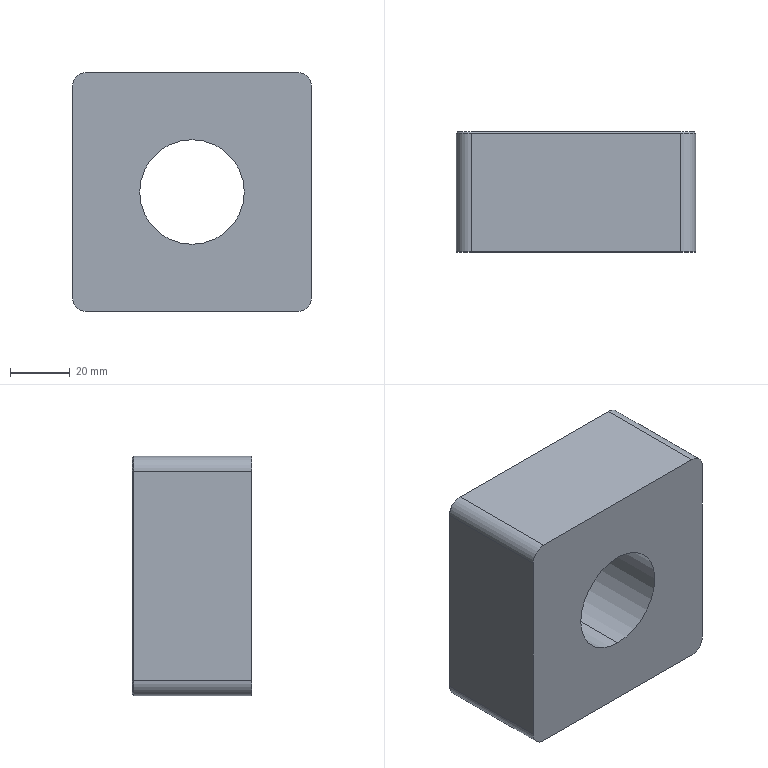Part | SolidWorks | features Chamfer 1, Extrusion 1, Fillet 1, HoleWzd 1 | 1 solid | 20 faces | box 80 x 40 x 80 mm | volume 216618 mm3 | plane 10 | cylinder 6 | cone 4 | commonest cylinder face diameters 10 x4 35 x2
STEP:
#1=CARTESIAN_POINT('',(0.,-25.,-17.5));
#2=VERTEX_POINT('',#1);
#3=CARTESIAN_POINT('',(0.,-25.,17.5));
#4=VERTEX_POINT('',#3);
#5=CARTESIAN_POINT('',(0.,-25.,0.));
#6=DIRECTION('',(0.,1.,0.));
#7=DIRECTION('',(0.,0.,1.));
#8=AXIS2_PLACEMENT_3D('',#5,#6,#7);
#9=CIRCLE('',#8,17.5);
#10=EDGE_CURVE('',#2,#4,#9,.T.);
#11=ORIENTED_EDGE('',*,*,#10,.F.);
#12=CARTESIAN_POINT('',(0.,15.,-17.5));
#13=VERTEX_POINT('',#12);
#14=CARTESIAN_POINT('',(0.,15.,-17.5));
#15=DIRECTION('',(0.,1.,0.));
#16=VECTOR('',#15,1000.);
#17=LINE('',#14,#16);
#18=EDGE_CURVE('',#2,#13,#17,.T.);
#19=ORIENTED_EDGE('',*,*,#18,.T.);
#20=CARTESIAN_POINT('',(0.,15.,17.5));
#21=VERTEX_POINT('',#20);
#22=CARTESIAN_POINT('',(0.,15.,0.));
#23=DIRECTION('',(0.,1.,0.));
#24=DIRECTION('',(0.,0.,1.));
#25=AXIS2_PLACEMENT_3D('',#22,#23,#24);
#26=CIRCLE('',#25,17.5);
#27=EDGE_CURVE('',#13,#21,#26,.T.);
#28=ORIENTED_EDGE('',*,*,#27,.T.);
#29=CARTESIAN_POINT('',(0.,15.,17.5));
#30=DIRECTION('',(0.,1.,0.));
#31=VECTOR('',#30,1000.);
#32=LINE('',#29,#31);
#33=EDGE_CURVE('',#4,#21,#32,.T.);
#34=ORIENTED_EDGE('',*,*,#33,.F.);
#35=EDGE_LOOP('',(#11,#19,#28,#34));
#36=FACE_OUTER_BOUND('',#35,.T.);
#37=CARTESIAN_POINT('',(0.,15.,0.));
#38=DIRECTION('',(0.,1.,0.));
#39=DIRECTION('',(0.,0.,1.));
#40=AXIS2_PLACEMENT_3D('',#37,#38,#39);
#41=CYLINDRICAL_SURFACE('',#40,17.5);
#42=ADVANCED_FACE('',(#36),#41,.F.);
#43=CARTESIAN_POINT('',(-40.,-25.,35.));
#44=VERTEX_POINT('',#43);
#45=CARTESIAN_POINT('',(-40.,14.5,35.));
#46=VERTEX_POINT('',#45);
#47=CARTESIAN_POINT('',(-40.,-25.,35.));
#48=DIRECTION('',(0.,1.,0.));
#49=VECTOR('',#48,1000.);
#50=LINE('',#47,#49);
#51=EDGE_CURVE('',#44,#46,#50,.T.);
#52=ORIENTED_EDGE('',*,*,#51,.T.);
#53=CARTESIAN_POINT('',(-40.,14.5,-35.));
#54=VERTEX_POINT('',#53);
#55=CARTESIAN_POINT('',(-40.,14.5,-40.));
#56=DIRECTION('',(0.,0.,-1.));
#57=VECTOR('',#56,1000.);
#58=LINE('',#55,#57);
#59=EDGE_CURVE('',#46,#54,#58,.T.);
#60=ORIENTED_EDGE('',*,*,#59,.T.);
#61=CARTESIAN_POINT('',(-40.,-25.,-35.));
#62=VERTEX_POINT('',#61);
#63=CARTESIAN_POINT('',(-40.,-25.,-35.));
#64=DIRECTION('',(0.,-1.,0.));
#65=VECTOR('',#64,1000.);
#66=LINE('',#63,#65);
#67=EDGE_CURVE('',#54,#62,#66,.T.);
#68=ORIENTED_EDGE('',*,*,#67,.T.);
#69=CARTESIAN_POINT('',(-40.,-25.,-40.));
#70=DIRECTION('',(0.,0.,1.));
#71=VECTOR('',#70,1000.);
#72=LINE('',#69,#71);
#73=EDGE_CURVE('',#62,#44,#72,.T.);
#74=ORIENTED_EDGE('',*,*,#73,.T.);
#75=EDGE_LOOP('',(#52,#60,#68,#74));
#76=FACE_OUTER_BOUND('',#75,.T.);
#77=CARTESIAN_POINT('',(-40.,-25.,-40.));
#78=DIRECTION('',(-1.,0.,0.));
#79=DIRECTION('',(0.,0.,1.));
#80=AXIS2_PLACEMENT_3D('',#77,#78,#79);
#81=PLANE('',#80);
#82=ADVANCED_FACE('',(#76),#81,.T.);
#83=CARTESIAN_POINT('',(-35.,-25.,-40.));
#84=VERTEX_POINT('',#83);
#85=CARTESIAN_POINT('',(-35.,14.5,-40.));
#86=VERTEX_POINT('',#85);
#87=CARTESIAN_POINT('',(-35.,-25.,-40.));
#88=DIRECTION('',(0.,1.,0.));
#89=VECTOR('',#88,1000.);
#90=LINE('',#87,#89);
#91=EDGE_CURVE('',#84,#86,#90,.T.);
#92=ORIENTED_EDGE('',*,*,#91,.T.);
#93=CARTESIAN_POINT('',(35.,14.5,-40.));
#94=VERTEX_POINT('',#93);
#95=CARTESIAN_POINT('',(40.,14.5,-40.));
#96=DIRECTION('',(1.,0.,0.));
#97=VECTOR('',#96,1000.);
#98=LINE('',#95,#97);
#99=EDGE_CURVE('',#86,#94,#98,.T.);
#100=ORIENTED_EDGE('',*,*,#99,.T.);
#101=CARTESIAN_POINT('',(35.,-25.,-40.));
#102=VERTEX_POINT('',#101);
#103=CARTESIAN_POINT('',(35.,-25.,-40.));
#104=DIRECTION('',(0.,-1.,0.));
#105=VECTOR('',#104,1000.);
#106=LINE('',#103,#105);
#107=EDGE_CURVE('',#94,#102,#106,.T.);
#108=ORIENTED_EDGE('',*,*,#107,.T.);
#109=CARTESIAN_POINT('',(40.,-25.,-40.));
#110=DIRECTION('',(-1.,0.,0.));
#111=VECTOR('',#110,1000.);
#112=LINE('',#109,#111);
#113=EDGE_CURVE('',#102,#84,#112,.T.);
#114=ORIENTED_EDGE('',*,*,#113,.T.);
#115=EDGE_LOOP('',(#92,#100,#108,#114));
#116=FACE_OUTER_BOUND('',#115,.T.);
#117=CARTESIAN_POINT('',(40.,-25.,-40.));
#118=DIRECTION('',(0.,0.,-1.));
#119=DIRECTION('',(-1.,0.,0.));
#120=AXIS2_PLACEMENT_3D('',#117,#118,#119);
#121=PLANE('',#120);
#122=ADVANCED_FACE('',(#116),#121,.T.);
#123=CARTESIAN_POINT('',(40.,-25.,-35.));
#124=VERTEX_POINT('',#123);
#125=CARTESIAN_POINT('',(40.,14.5,-35.));
#126=VERTEX_POINT('',#125);
#127=CARTESIAN_POINT('',(40.,-25.,-35.));
#128=DIRECTION('',(0.,1.,0.));
#129=VECTOR('',#128,1000.);
#130=LINE('',#127,#129);
#131=EDGE_CURVE('',#124,#126,#130,.T.);
#132=ORIENTED_EDGE('',*,*,#131,.T.);
#133=CARTESIAN_POINT('',(40.,14.5,35.));
#134=VERTEX_POINT('',#133);
#135=CARTESIAN_POINT('',(40.,14.5,40.));
#136=DIRECTION('',(0.,0.,1.));
#137=VECTOR('',#136,1000.);
#138=LINE('',#135,#137);
#139=EDGE_CURVE('',#126,#134,#138,.T.);
#140=ORIENTED_EDGE('',*,*,#139,.T.);
#141=CARTESIAN_POINT('',(40.,-25.,35.));
#142=VERTEX_POINT('',#141);
#143=CARTESIAN_POINT('',(40.,-25.,35.));
#144=DIRECTION('',(0.,-1.,0.));
#145=VECTOR('',#144,1000.);
#146=LINE('',#143,#145);
#147=EDGE_CURVE('',#134,#142,#146,.T.);
#148=ORIENTED_EDGE('',*,*,#147,.T.);
#149=CARTESIAN_POINT('',(40.,-25.,40.));
#150=DIRECTION('',(0.,0.,-1.));
#151=VECTOR('',#150,1000.);
#152=LINE('',#149,#151);
#153=EDGE_CURVE('',#142,#124,#152,.T.);
#154=ORIENTED_EDGE('',*,*,#153,.T.);
#155=EDGE_LOOP('',(#132,#140,#148,#154));
#156=FACE_OUTER_BOUND('',#155,.T.);
#157=CARTESIAN_POINT('',(40.,-25.,40.));
#158=DIRECTION('',(1.,0.,0.));
#159=DIRECTION('',(0.,0.,-1.));
#160=AXIS2_PLACEMENT_3D('',#157,#158,#159);
#161=PLANE('',#160);
#162=ADVANCED_FACE('',(#156),#161,.T.);
#163=CARTESIAN_POINT('',(35.,-25.,40.));
#164=VERTEX_POINT('',#163);
#165=CARTESIAN_POINT('',(35.,14.5,40.));
#166=VERTEX_POINT('',#165);
#167=CARTESIAN_POINT('',(35.,-25.,40.));
#168=DIRECTION('',(0.,1.,0.));
#169=VECTOR('',#168,1000.);
#170=LINE('',#167,#169);
#171=EDGE_CURVE('',#164,#166,#170,.T.);
#172=ORIENTED_EDGE('',*,*,#171,.T.);
#173=CARTESIAN_POINT('',(-35.,14.5,40.));
#174=VERTEX_POINT('',#173);
#175=CARTESIAN_POINT('',(-40.,14.5,40.));
#176=DIRECTION('',(-1.,0.,0.));
#177=VECTOR('',#176,1000.);
#178=LINE('',#175,#177);
#179=EDGE_CURVE('',#166,#174,#178,.T.);
#180=ORIENTED_EDGE('',*,*,#179,.T.);
#181=CARTESIAN_POINT('',(-35.,-25.,40.));
#182=VERTEX_POINT('',#181);
#183=CARTESIAN_POINT('',(-35.,-25.,40.));
#184=DIRECTION('',(0.,-1.,0.));
#185=VECTOR('',#184,1000.);
#186=LINE('',#183,#185);
#187=EDGE_CURVE('',#174,#182,#186,.T.);
#188=ORIENTED_EDGE('',*,*,#187,.T.);
#189=CARTESIAN_POINT('',(-40.,-25.,40.));
#190=DIRECTION('',(1.,0.,0.));
#191=VECTOR('',#190,1000.);
#192=LINE('',#189,#191);
#193=EDGE_CURVE('',#182,#164,#192,.T.);
#194=ORIENTED_EDGE('',*,*,#193,.T.);
#195=EDGE_LOOP('',(#172,#180,#188,#194));
#196=FACE_OUTER_BOUND('',#195,.T.);
#197=CARTESIAN_POINT('',(-40.,-25.,40.));
#198=DIRECTION('',(0.,0.,1.));
#199=DIRECTION('',(1.,0.,0.));
#200=AXIS2_PLACEMENT_3D('',#197,#198,#199);
#201=PLANE('',#200);
#202=ADVANCED_FACE('',(#196),#201,.T.);
#203=CARTESIAN_POINT('',(0.,-25.,0.));
#204=DIRECTION('',(0.,1.,0.));
#205=DIRECTION('',(0.,0.,1.));
#206=AXIS2_PLACEMENT_3D('',#203,#204,#205);
#207=CIRCLE('',#206,17.5);
#208=EDGE_CURVE('',#4,#2,#207,.T.);
#209=ORIENTED_EDGE('',*,*,#208,.T.);
#210=ORIENTED_EDGE('',*,*,#10,.T.);
#211=EDGE_LOOP('',(#209,#210));
#212=FACE_BOUND('',#211,.T.);
#213=ORIENTED_EDGE('',*,*,#153,.F.);
#214=CARTESIAN_POINT('',(35.,-25.,35.));
#215=DIRECTION('',(0.,-1.,0.));
#216=DIRECTION('',(0.,0.,1.));
#217=AXIS2_PLACEMENT_3D('',#214,#215,#216);
#218=CIRCLE('',#217,5.);
#219=EDGE_CURVE('',#142,#164,#218,.T.);
#220=ORIENTED_EDGE('',*,*,#219,.T.);
#221=ORIENTED_EDGE('',*,*,#193,.F.);
#222=CARTESIAN_POINT('',(-35.,-25.,35.));
#223=DIRECTION('',(0.,-1.,0.));
#224=DIRECTION('',(0.,0.,1.));
#225=AXIS2_PLACEMENT_3D('',#222,#223,#224);
#226=CIRCLE('',#225,5.);
#227=EDGE_CURVE('',#182,#44,#226,.T.);
#228=ORIENTED_EDGE('',*,*,#227,.T.);
#229=ORIENTED_EDGE('',*,*,#73,.F.);
#230=CARTESIAN_POINT('',(-35.,-25.,-35.));
#231=DIRECTION('',(0.,-1.,0.));
#232=DIRECTION('',(0.,0.,1.));
#233=AXIS2_PLACEMENT_3D('',#230,#231,#232);
#234=CIRCLE('',#233,5.);
#235=EDGE_CURVE('',#62,#84,#234,.T.);
#236=ORIENTED_EDGE('',*,*,#235,.T.);
#237=ORIENTED_EDGE('',*,*,#113,.F.);
#238=CARTESIAN_POINT('',(35.,-25.,-35.));
#239=DIRECTION('',(0.,-1.,0.));
#240=DIRECTION('',(0.,0.,1.));
#241=AXIS2_PLACEMENT_3D('',#238,#239,#240);
#242=CIRCLE('',#241,5.);
#243=EDGE_CURVE('',#102,#124,#242,.T.);
#244=ORIENTED_EDGE('',*,*,#243,.T.);
#245=EDGE_LOOP('',(#213,#220,#221,#228,#229,#236,#237,#244));
#246=FACE_OUTER_BOUND('',#245,.T.);
#247=CARTESIAN_POINT('',(0.,-25.,0.));
#248=DIRECTION('',(0.,1.,0.));
#249=DIRECTION('',(0.,0.,1.));
#250=AXIS2_PLACEMENT_3D('',#247,#248,#249);
#251=PLANE('',#250);
#252=ADVANCED_FACE('',(#212,#246),#251,.F.);
#253=CARTESIAN_POINT('',(39.5,15.,-35.));
#254=VERTEX_POINT('',#253);
#255=CARTESIAN_POINT('',(35.,15.,-39.5));
#256=VERTEX_POINT('',#255);
#257=CARTESIAN_POINT('',(35.,15.,-35.));
#258=DIRECTION('',(0.,1.,0.));
#259=DIRECTION('',(0.,0.,1.));
#260=AXIS2_PLACEMENT_3D('',#257,#258,#259);
#261=CIRCLE('',#260,4.5);
#262=EDGE_CURVE('',#254,#256,#261,.T.);
#263=ORIENTED_EDGE('',*,*,#262,.T.);
#264=CARTESIAN_POINT('',(-35.,15.,-39.5));
#265=VERTEX_POINT('',#264);
#266=CARTESIAN_POINT('',(0.,15.,-39.5));
#267=DIRECTION('',(-1.,0.,0.));
#268=VECTOR('',#267,1000.);
#269=LINE('',#266,#268);
#270=EDGE_CURVE('',#256,#265,#269,.T.);
#271=ORIENTED_EDGE('',*,*,#270,.T.);
#272=CARTESIAN_POINT('',(-39.5,15.,-35.));
#273=VERTEX_POINT('',#272);
#274=CARTESIAN_POINT('',(-35.,15.,-35.));
#275=DIRECTION('',(0.,1.,0.));
#276=DIRECTION('',(0.,0.,1.));
#277=AXIS2_PLACEMENT_3D('',#274,#275,#276);
#278=CIRCLE('',#277,4.5);
#279=EDGE_CURVE('',#265,#273,#278,.T.);
#280=ORIENTED_EDGE('',*,*,#279,.T.);
#281=CARTESIAN_POINT('',(-39.5,15.,35.));
#282=VERTEX_POINT('',#281);
#283=CARTESIAN_POINT('',(-39.5,15.,0.));
#284=DIRECTION('',(0.,0.,1.));
#285=VECTOR('',#284,1000.);
#286=LINE('',#283,#285);
#287=EDGE_CURVE('',#273,#282,#286,.T.);
#288=ORIENTED_EDGE('',*,*,#287,.T.);
#289=CARTESIAN_POINT('',(-35.,15.,39.5));
#290=VERTEX_POINT('',#289);
#291=CARTESIAN_POINT('',(-35.,15.,35.));
#292=DIRECTION('',(0.,1.,0.));
#293=DIRECTION('',(0.,0.,1.));
#294=AXIS2_PLACEMENT_3D('',#291,#292,#293);
#295=CIRCLE('',#294,4.5);
#296=EDGE_CURVE('',#282,#290,#295,.T.);
#297=ORIENTED_EDGE('',*,*,#296,.T.);
#298=CARTESIAN_POINT('',(35.,15.,39.5));
#299=VERTEX_POINT('',#298);
#300=CARTESIAN_POINT('',(0.,15.,39.5));
#301=DIRECTION('',(1.,0.,0.));
#302=VECTOR('',#301,1000.);
#303=LINE('',#300,#302);
#304=EDGE_CURVE('',#290,#299,#303,.T.);
#305=ORIENTED_EDGE('',*,*,#304,.T.);
#306=CARTESIAN_POINT('',(39.5,15.,35.));
#307=VERTEX_POINT('',#306);
#308=CARTESIAN_POINT('',(35.,15.,35.));
#309=DIRECTION('',(0.,1.,0.));
#310=DIRECTION('',(0.,0.,1.));
#311=AXIS2_PLACEMENT_3D('',#308,#309,#310);
#312=CIRCLE('',#311,4.5);
#313=EDGE_CURVE('',#299,#307,#312,.T.);
#314=ORIENTED_EDGE('',*,*,#313,.T.);
#315=CARTESIAN_POINT('',(39.5,15.,0.));
#316=DIRECTION('',(0.,0.,-1.));
#317=VECTOR('',#316,1000.);
#318=LINE('',#315,#317);
#319=EDGE_CURVE('',#307,#254,#318,.T.);
#320=ORIENTED_EDGE('',*,*,#319,.T.);
#321=EDGE_LOOP('',(#263,#271,#280,#288,#297,#305,#314,#320));
#322=FACE_OUTER_BOUND('',#321,.T.);
#323=CARTESIAN_POINT('',(0.,15.,0.));
#324=DIRECTION('',(0.,1.,0.));
#325=DIRECTION('',(0.,0.,1.));
#326=AXIS2_PLACEMENT_3D('',#323,#324,#325);
#327=CIRCLE('',#326,17.5);
#328=EDGE_CURVE('',#21,#13,#327,.T.);
#329=ORIENTED_EDGE('',*,*,#328,.F.);
#330=ORIENTED_EDGE('',*,*,#27,.F.);
#331=EDGE_LOOP('',(#329,#330));
#332=FACE_BOUND('',#331,.T.);
#333=CARTESIAN_POINT('',(0.,15.,0.));
#334=DIRECTION('',(0.,1.,0.));
#335=DIRECTION('',(0.,0.,1.));
#336=AXIS2_PLACEMENT_3D('',#333,#334,#335);
#337=PLANE('',#336);
#338=ADVANCED_FACE('',(#322,#332),#337,.T.);
#339=ORIENTED_EDGE('',*,*,#18,.F.);
#340=ORIENTED_EDGE('',*,*,#208,.F.);
#341=ORIENTED_EDGE('',*,*,#33,.T.);
#342=ORIENTED_EDGE('',*,*,#328,.T.);
#343=EDGE_LOOP('',(#339,#340,#341,#342));
#344=FACE_OUTER_BOUND('',#343,.T.);
#345=CARTESIAN_POINT('',(0.,15.,0.));
#346=DIRECTION('',(0.,1.,0.));
#347=DIRECTION('',(0.,0.,1.));
#348=AXIS2_PLACEMENT_3D('',#345,#346,#347);
#349=CYLINDRICAL_SURFACE('',#348,17.5);
#350=ADVANCED_FACE('',(#344),#349,.F.);
#351=ORIENTED_EDGE('',*,*,#147,.F.);
#352=CARTESIAN_POINT('',(35.,14.5,35.));
#353=DIRECTION('',(0.,-1.,0.));
#354=DIRECTION('',(0.,0.,1.));
#355=AXIS2_PLACEMENT_3D('',#352,#353,#354);
#356=CIRCLE('',#355,5.);
#357=EDGE_CURVE('',#134,#166,#356,.T.);
#358=ORIENTED_EDGE('',*,*,#357,.T.);
#359=ORIENTED_EDGE('',*,*,#171,.F.);
#360=ORIENTED_EDGE('',*,*,#219,.F.);
#361=EDGE_LOOP('',(#351,#358,#359,#360));
#362=FACE_OUTER_BOUND('',#361,.T.);
#363=CARTESIAN_POINT('',(35.,-25.,35.));
#364=DIRECTION('',(0.,1.,0.));
#365=DIRECTION('',(0.,0.,1.));
#366=AXIS2_PLACEMENT_3D('',#363,#364,#365);
#367=CYLINDRICAL_SURFACE('',#366,5.);
#368=ADVANCED_FACE('',(#362),#367,.T.);
#369=ORIENTED_EDGE('',*,*,#187,.F.);
#370=CARTESIAN_POINT('',(-35.,14.5,35.));
#371=DIRECTION('',(0.,-1.,0.));
#372=DIRECTION('',(0.,0.,1.));
#373=AXIS2_PLACEMENT_3D('',#370,#371,#372);
#374=CIRCLE('',#373,5.);
#375=EDGE_CURVE('',#174,#46,#374,.T.);
#376=ORIENTED_EDGE('',*,*,#375,.T.);
#377=ORIENTED_EDGE('',*,*,#51,.F.);
#378=ORIENTED_EDGE('',*,*,#227,.F.);
#379=EDGE_LOOP('',(#369,#376,#377,#378));
#380=FACE_OUTER_BOUND('',#379,.T.);
#381=CARTESIAN_POINT('',(-35.,-25.,35.));
#382=DIRECTION('',(0.,1.,0.));
#383=DIRECTION('',(0.,0.,1.));
#384=AXIS2_PLACEMENT_3D('',#381,#382,#383);
#385=CYLINDRICAL_SURFACE('',#384,5.);
#386=ADVANCED_FACE('',(#380),#385,.T.);
#387=ORIENTED_EDGE('',*,*,#107,.F.);
#388=CARTESIAN_POINT('',(35.,14.5,-35.));
#389=DIRECTION('',(0.,-1.,0.));
#390=DIRECTION('',(0.,0.,1.));
#391=AXIS2_PLACEMENT_3D('',#388,#389,#390);
#392=CIRCLE('',#391,5.);
#393=EDGE_CURVE('',#94,#126,#392,.T.);
#394=ORIENTED_EDGE('',*,*,#393,.T.);
#395=ORIENTED_EDGE('',*,*,#131,.F.);
#396=ORIENTED_EDGE('',*,*,#243,.F.);
#397=EDGE_LOOP('',(#387,#394,#395,#396));
#398=FACE_OUTER_BOUND('',#397,.T.);
#399=CARTESIAN_POINT('',(35.,-25.,-35.));
#400=DIRECTION('',(0.,1.,0.));
#401=DIRECTION('',(0.,0.,1.));
#402=AXIS2_PLACEMENT_3D('',#399,#400,#401);
#403=CYLINDRICAL_SURFACE('',#402,5.);
#404=ADVANCED_FACE('',(#398),#403,.T.);
#405=ORIENTED_EDGE('',*,*,#67,.F.);
#406=CARTESIAN_POINT('',(-35.,14.5,-35.));
#407=DIRECTION('',(0.,-1.,0.));
#408=DIRECTION('',(0.,0.,1.));
#409=AXIS2_PLACEMENT_3D('',#406,#407,#408);
#410=CIRCLE('',#409,5.);
#411=EDGE_CURVE('',#54,#86,#410,.T.);
#412=ORIENTED_EDGE('',*,*,#411,.T.);
#413=ORIENTED_EDGE('',*,*,#91,.F.);
#414=ORIENTED_EDGE('',*,*,#235,.F.);
#415=EDGE_LOOP('',(#405,#412,#413,#414));
#416=FACE_OUTER_BOUND('',#415,.T.);
#417=CARTESIAN_POINT('',(-35.,-25.,-35.));
#418=DIRECTION('',(0.,1.,0.));
#419=DIRECTION('',(0.,0.,1.));
#420=AXIS2_PLACEMENT_3D('',#417,#418,#419);
#421=CYLINDRICAL_SURFACE('',#420,5.);
#422=ADVANCED_FACE('',(#416),#421,.T.);
#423=CARTESIAN_POINT('',(-35.,14.5,40.));
#424=DIRECTION('',(0.,0.7071,-0.7071));
#425=VECTOR('',#424,1000.);
#426=LINE('',#423,#425);
#427=EDGE_CURVE('',#174,#290,#426,.T.);
#428=ORIENTED_EDGE('',*,*,#427,.F.);
#429=ORIENTED_EDGE('',*,*,#179,.F.);
#430=CARTESIAN_POINT('',(35.,15.,39.5));
#431=DIRECTION('',(0.,-0.7071,0.7071));
#432=VECTOR('',#431,1000.);
#433=LINE('',#430,#432);
#434=EDGE_CURVE('',#299,#166,#433,.T.);
#435=ORIENTED_EDGE('',*,*,#434,.F.);
#436=ORIENTED_EDGE('',*,*,#304,.F.);
#437=EDGE_LOOP('',(#428,#429,#435,#436));
#438=FACE_OUTER_BOUND('',#437,.T.);
#439=CARTESIAN_POINT('',(0.,15.,39.5));
#440=DIRECTION('',(0.,-0.7071,-0.7071));
#441=DIRECTION('',(1.,0.,0.));
#442=AXIS2_PLACEMENT_3D('',#439,#440,#441);
#443=PLANE('',#442);
#444=ADVANCED_FACE('',(#438),#443,.F.);
#445=ORIENTED_EDGE('',*,*,#434,.T.);
#446=ORIENTED_EDGE('',*,*,#357,.F.);
#447=CARTESIAN_POINT('',(39.5,15.,35.));
#448=DIRECTION('',(0.7071,-0.7071,0.));
#449=VECTOR('',#448,1000.);
#450=LINE('',#447,#449);
#451=EDGE_CURVE('',#307,#134,#450,.T.);
#452=ORIENTED_EDGE('',*,*,#451,.F.);
#453=ORIENTED_EDGE('',*,*,#313,.F.);
#454=EDGE_LOOP('',(#445,#446,#452,#453));
#455=FACE_OUTER_BOUND('',#454,.T.);
#456=CARTESIAN_POINT('',(35.,15.,35.));
#457=DIRECTION('',(0.,-1.,0.));
#458=DIRECTION('',(0.,0.,-1.));
#459=AXIS2_PLACEMENT_3D('',#456,#457,#458);
#460=CONICAL_SURFACE('',#459,4.5,0.7854);
#461=ADVANCED_FACE('',(#455),#460,.T.);
#462=ORIENTED_EDGE('',*,*,#427,.T.);
#463=ORIENTED_EDGE('',*,*,#296,.F.);
#464=CARTESIAN_POINT('',(-40.,14.5,35.));
#465=DIRECTION('',(0.7071,0.7071,0.));
#466=VECTOR('',#465,1000.);
#467=LINE('',#464,#466);
#468=EDGE_CURVE('',#46,#282,#467,.T.);
#469=ORIENTED_EDGE('',*,*,#468,.F.);
#470=ORIENTED_EDGE('',*,*,#375,.F.);
#471=EDGE_LOOP('',(#462,#463,#469,#470));
#472=FACE_OUTER_BOUND('',#471,.T.);
#473=CARTESIAN_POINT('',(-35.,15.,35.));
#474=DIRECTION('',(0.,-1.,0.));
#475=DIRECTION('',(0.,0.,-1.));
#476=AXIS2_PLACEMENT_3D('',#473,#474,#475);
#477=CONICAL_SURFACE('',#476,4.5,0.7854);
#478=ADVANCED_FACE('',(#472),#477,.T.);
#479=ORIENTED_EDGE('',*,*,#451,.T.);
#480=ORIENTED_EDGE('',*,*,#139,.F.);
#481=CARTESIAN_POINT('',(39.5,15.,-35.));
#482=DIRECTION('',(0.7071,-0.7071,0.));
#483=VECTOR('',#482,1000.);
#484=LINE('',#481,#483);
#485=EDGE_CURVE('',#254,#126,#484,.T.);
#486=ORIENTED_EDGE('',*,*,#485,.F.);
#487=ORIENTED_EDGE('',*,*,#319,.F.);
#488=EDGE_LOOP('',(#479,#480,#486,#487));
#489=FACE_OUTER_BOUND('',#488,.T.);
#490=CARTESIAN_POINT('',(39.5,15.,0.));
#491=DIRECTION('',(-0.7071,-0.7071,0.));
#492=DIRECTION('',(0.,0.,-1.));
#493=AXIS2_PLACEMENT_3D('',#490,#491,#492);
#494=PLANE('',#493);
#495=ADVANCED_FACE('',(#489),#494,.F.);
#496=ORIENTED_EDGE('',*,*,#468,.T.);
#497=ORIENTED_EDGE('',*,*,#287,.F.);
#498=CARTESIAN_POINT('',(-40.,14.5,-35.));
#499=DIRECTION('',(0.7071,0.7071,0.));
#500=VECTOR('',#499,1000.);
#501=LINE('',#498,#500);
#502=EDGE_CURVE('',#54,#273,#501,.T.);
#503=ORIENTED_EDGE('',*,*,#502,.F.);
#504=ORIENTED_EDGE('',*,*,#59,.F.);
#505=EDGE_LOOP('',(#496,#497,#503,#504));
#506=FACE_OUTER_BOUND('',#505,.T.);
#507=CARTESIAN_POINT('',(-39.5,15.,0.));
#508=DIRECTION('',(0.7071,-0.7071,0.));
#509=DIRECTION('',(0.,0.,1.));
#510=AXIS2_PLACEMENT_3D('',#507,#508,#509);
#511=PLANE('',#510);
#512=ADVANCED_FACE('',(#506),#511,.F.);
#513=ORIENTED_EDGE('',*,*,#485,.T.);
#514=ORIENTED_EDGE('',*,*,#393,.F.);
#515=CARTESIAN_POINT('',(35.,15.,-39.5));
#516=DIRECTION('',(0.,-0.7071,-0.7071));
#517=VECTOR('',#516,1000.);
#518=LINE('',#515,#517);
#519=EDGE_CURVE('',#256,#94,#518,.T.);
#520=ORIENTED_EDGE('',*,*,#519,.F.);
#521=ORIENTED_EDGE('',*,*,#262,.F.);
#522=EDGE_LOOP('',(#513,#514,#520,#521));
#523=FACE_OUTER_BOUND('',#522,.T.);
#524=CARTESIAN_POINT('',(35.,15.,-35.));
#525=DIRECTION('',(0.,-1.,0.));
#526=DIRECTION('',(0.,0.,-1.));
#527=AXIS2_PLACEMENT_3D('',#524,#525,#526);
#528=CONICAL_SURFACE('',#527,4.5,0.7854);
#529=ADVANCED_FACE('',(#523),#528,.T.);
#530=ORIENTED_EDGE('',*,*,#502,.T.);
#531=ORIENTED_EDGE('',*,*,#279,.F.);
#532=CARTESIAN_POINT('',(-35.,14.5,-40.));
#533=DIRECTION('',(0.,0.7071,0.7071));
#534=VECTOR('',#533,1000.);
#535=LINE('',#532,#534);
#536=EDGE_CURVE('',#86,#265,#535,.T.);
#537=ORIENTED_EDGE('',*,*,#536,.F.);
#538=ORIENTED_EDGE('',*,*,#411,.F.);
#539=EDGE_LOOP('',(#530,#531,#537,#538));
#540=FACE_OUTER_BOUND('',#539,.T.);
#541=CARTESIAN_POINT('',(-35.,15.,-35.));
#542=DIRECTION('',(0.,-1.,0.));
#543=DIRECTION('',(0.,0.,-1.));
#544=AXIS2_PLACEMENT_3D('',#541,#542,#543);
#545=CONICAL_SURFACE('',#544,4.5,0.7854);
#546=ADVANCED_FACE('',(#540),#545,.T.);
#547=ORIENTED_EDGE('',*,*,#519,.T.);
#548=ORIENTED_EDGE('',*,*,#99,.F.);
#549=ORIENTED_EDGE('',*,*,#536,.T.);
#550=ORIENTED_EDGE('',*,*,#270,.F.);
#551=EDGE_LOOP('',(#547,#548,#549,#550));
#552=FACE_OUTER_BOUND('',#551,.T.);
#553=CARTESIAN_POINT('',(0.,15.,-39.5));
#554=DIRECTION('',(0.,-0.7071,0.7071));
#555=DIRECTION('',(-1.,0.,0.));
#556=AXIS2_PLACEMENT_3D('',#553,#554,#555);
#557=PLANE('',#556);
#558=ADVANCED_FACE('',(#552),#557,.F.);
#559=CLOSED_SHELL('',(#42,#82,#122,#162,#202,#252,#338,#350,#368,#386,#404,#422,#444,#461,#478,#495,#512,#529,#546,#558));
#560=MANIFOLD_SOLID_BREP('',#559);
#561=CARTESIAN_POINT('',(0.,0.,0.));
#562=DIRECTION('',(0.,0.,1.));
#563=DIRECTION('',(1.,0.,0.));
#564=AXIS2_PLACEMENT_3D('',#561,#562,#563);
#565=(LENGTH_UNIT()NAMED_UNIT(*)SI_UNIT(.MILLI.,.METRE.));
#566=UNCERTAINTY_MEASURE_WITH_UNIT(LENGTH_MEASURE(0.00001),#565,'','');
#567=(NAMED_UNIT(*)PLANE_ANGLE_UNIT()SI_UNIT($,.RADIAN.));
#568=(NAMED_UNIT(*)SI_UNIT($,.STERADIAN.)SOLID_ANGLE_UNIT());
#569=(GEOMETRIC_REPRESENTATION_CONTEXT(3)GLOBAL_UNCERTAINTY_ASSIGNED_CONTEXT((#566))GLOBAL_UNIT_ASSIGNED_CONTEXT((#565,#567,#568))REPRESENTATION_CONTEXT('',''));
#570=ADVANCED_BREP_SHAPE_REPRESENTATION('',(#560,#564),#569);